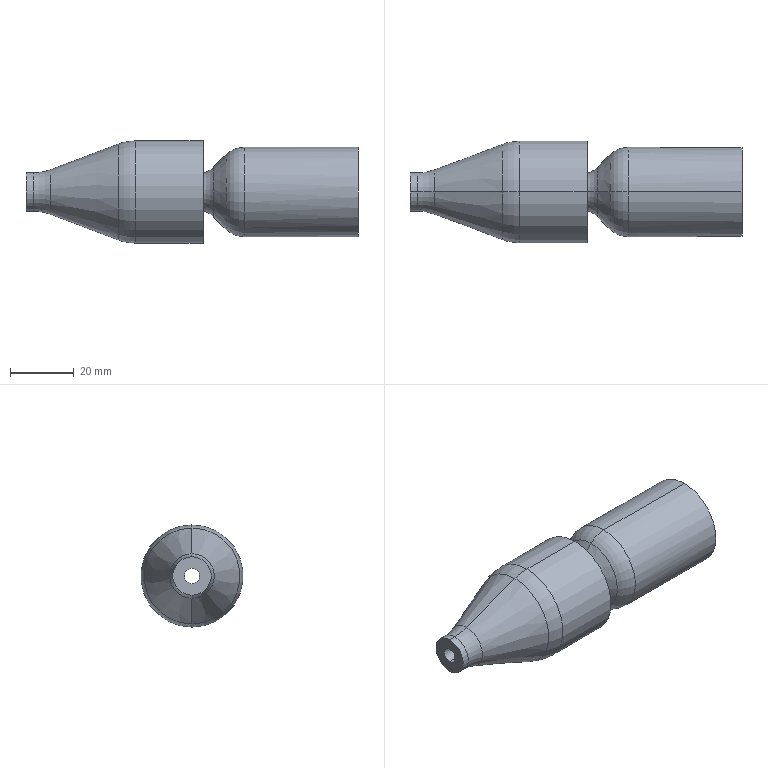Part | NX | features BREP 1 | 1 solid | 62 faces | box 104 x 32 x 32 mm | volume 43444 mm3 | torus 30 | cylinder 16 | plane 12 | cone 4 | commonest cylinder face diameters 4.76 x2 11 x2 12 x2 13 x2 20 x2 21 x2